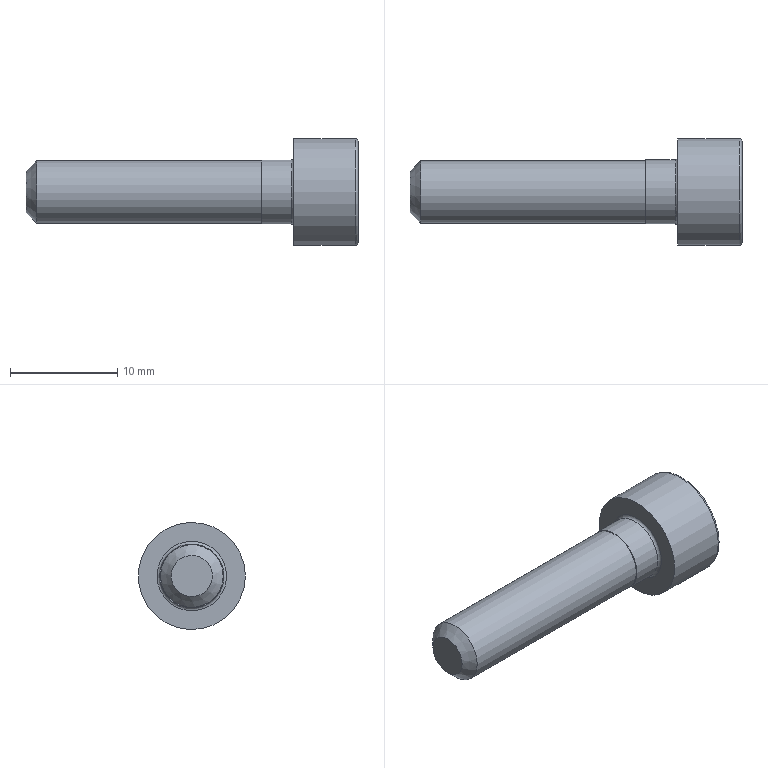Part | STEP file | PARAFUSO M6x25 - DIN_912 | 1 solid | 24 faces | box 31 x 10 x 10 mm | volume 1061 mm3 | plane 11 | cylinder 9 | torus 2 | cone 2 | commonest cylinder face diameters 5.723 x6 5.854 x1 6 x1 10 x1